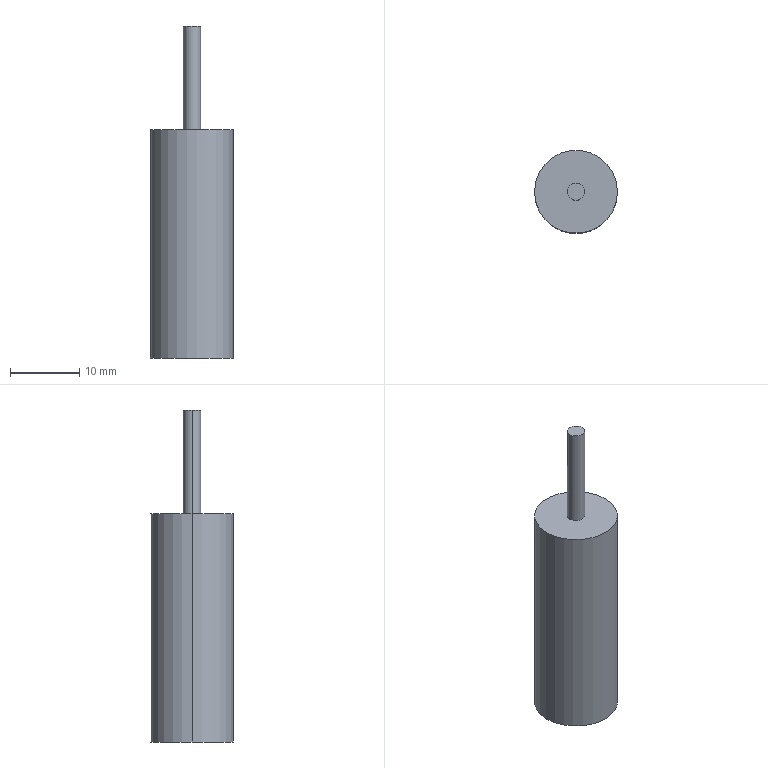Part | SolidWorks | features ICE 2 | 1 solid | 7 faces | box 12 x 12 x 48 mm | volume 3806 mm3 | cylinder 4 | plane 3 | commonest cylinder face diameters 2.5 x2 12 x2
STEP:
#1=CARTESIAN_POINT('',(1.25,0.,48.));
#2=VERTEX_POINT('',#1);
#3=CARTESIAN_POINT('',(-1.25,0.,48.));
#4=VERTEX_POINT('',#3);
#5=CARTESIAN_POINT('',(0.,0.,48.));
#6=DIRECTION('',(0.,0.,1.));
#7=DIRECTION('',(1.,0.,0.));
#8=AXIS2_PLACEMENT_3D('',#5,#6,#7);
#9=CIRCLE('',#8,1.25);
#10=EDGE_CURVE('',#2,#4,#9,.T.);
#11=ORIENTED_EDGE('',*,*,#10,.F.);
#12=CARTESIAN_POINT('',(1.25,0.,33.));
#13=VERTEX_POINT('',#12);
#14=CARTESIAN_POINT('',(1.25,0.,48.));
#15=DIRECTION('',(0.,0.,-1.));
#16=VECTOR('',#15,1000.);
#17=LINE('',#14,#16);
#18=EDGE_CURVE('',#2,#13,#17,.T.);
#19=ORIENTED_EDGE('',*,*,#18,.T.);
#20=CARTESIAN_POINT('',(-1.25,0.,33.));
#21=VERTEX_POINT('',#20);
#22=CARTESIAN_POINT('',(0.,0.,33.));
#23=DIRECTION('',(0.,0.,1.));
#24=DIRECTION('',(1.,0.,0.));
#25=AXIS2_PLACEMENT_3D('',#22,#23,#24);
#26=CIRCLE('',#25,1.25);
#27=EDGE_CURVE('',#13,#21,#26,.T.);
#28=ORIENTED_EDGE('',*,*,#27,.T.);
#29=CARTESIAN_POINT('',(-1.25,0.,48.));
#30=DIRECTION('',(0.,0.,-1.));
#31=VECTOR('',#30,1000.);
#32=LINE('',#29,#31);
#33=EDGE_CURVE('',#4,#21,#32,.T.);
#34=ORIENTED_EDGE('',*,*,#33,.F.);
#35=EDGE_LOOP('',(#11,#19,#28,#34));
#36=FACE_OUTER_BOUND('',#35,.T.);
#37=CARTESIAN_POINT('',(0.,0.,48.));
#38=DIRECTION('',(0.,0.,-1.));
#39=DIRECTION('',(-1.,0.,0.));
#40=AXIS2_PLACEMENT_3D('',#37,#38,#39);
#41=CYLINDRICAL_SURFACE('',#40,1.25);
#42=ADVANCED_FACE('',(#36),#41,.T.);
#43=CARTESIAN_POINT('',(6.,0.,33.));
#44=VERTEX_POINT('',#43);
#45=CARTESIAN_POINT('',(-6.,0.,33.));
#46=VERTEX_POINT('',#45);
#47=CARTESIAN_POINT('',(0.,0.,33.));
#48=DIRECTION('',(0.,0.,1.));
#49=DIRECTION('',(1.,0.,0.));
#50=AXIS2_PLACEMENT_3D('',#47,#48,#49);
#51=CIRCLE('',#50,6.);
#52=EDGE_CURVE('',#44,#46,#51,.T.);
#53=ORIENTED_EDGE('',*,*,#52,.F.);
#54=CARTESIAN_POINT('',(6.,0.,0.));
#55=VERTEX_POINT('',#54);
#56=CARTESIAN_POINT('',(6.,0.,33.));
#57=DIRECTION('',(0.,0.,-1.));
#58=VECTOR('',#57,1000.);
#59=LINE('',#56,#58);
#60=EDGE_CURVE('',#44,#55,#59,.T.);
#61=ORIENTED_EDGE('',*,*,#60,.T.);
#62=CARTESIAN_POINT('',(-6.,0.,0.));
#63=VERTEX_POINT('',#62);
#64=CARTESIAN_POINT('',(0.,0.,0.));
#65=DIRECTION('',(0.,0.,1.));
#66=DIRECTION('',(1.,0.,0.));
#67=AXIS2_PLACEMENT_3D('',#64,#65,#66);
#68=CIRCLE('',#67,6.);
#69=EDGE_CURVE('',#55,#63,#68,.T.);
#70=ORIENTED_EDGE('',*,*,#69,.T.);
#71=CARTESIAN_POINT('',(-6.,0.,33.));
#72=DIRECTION('',(0.,0.,-1.));
#73=VECTOR('',#72,1000.);
#74=LINE('',#71,#73);
#75=EDGE_CURVE('',#46,#63,#74,.T.);
#76=ORIENTED_EDGE('',*,*,#75,.F.);
#77=EDGE_LOOP('',(#53,#61,#70,#76));
#78=FACE_OUTER_BOUND('',#77,.T.);
#79=CARTESIAN_POINT('',(0.,0.,33.));
#80=DIRECTION('',(0.,0.,-1.));
#81=DIRECTION('',(-1.,0.,0.));
#82=AXIS2_PLACEMENT_3D('',#79,#80,#81);
#83=CYLINDRICAL_SURFACE('',#82,6.);
#84=ADVANCED_FACE('',(#78),#83,.T.);
#85=CARTESIAN_POINT('',(0.,0.,33.));
#86=DIRECTION('',(0.,0.,1.));
#87=DIRECTION('',(1.,0.,0.));
#88=AXIS2_PLACEMENT_3D('',#85,#86,#87);
#89=CIRCLE('',#88,6.);
#90=EDGE_CURVE('',#46,#44,#89,.T.);
#91=ORIENTED_EDGE('',*,*,#90,.T.);
#92=ORIENTED_EDGE('',*,*,#52,.T.);
#93=EDGE_LOOP('',(#91,#92));
#94=FACE_OUTER_BOUND('',#93,.T.);
#95=CARTESIAN_POINT('',(0.,0.,33.));
#96=DIRECTION('',(0.,0.,1.));
#97=DIRECTION('',(1.,0.,0.));
#98=AXIS2_PLACEMENT_3D('',#95,#96,#97);
#99=CIRCLE('',#98,1.25);
#100=EDGE_CURVE('',#21,#13,#99,.T.);
#101=ORIENTED_EDGE('',*,*,#100,.F.);
#102=ORIENTED_EDGE('',*,*,#27,.F.);
#103=EDGE_LOOP('',(#101,#102));
#104=FACE_BOUND('',#103,.T.);
#105=CARTESIAN_POINT('',(0.,0.,33.));
#106=DIRECTION('',(0.,0.,1.));
#107=DIRECTION('',(1.,0.,0.));
#108=AXIS2_PLACEMENT_3D('',#105,#106,#107);
#109=PLANE('',#108);
#110=ADVANCED_FACE('',(#94,#104),#109,.T.);
#111=ORIENTED_EDGE('',*,*,#60,.F.);
#112=ORIENTED_EDGE('',*,*,#90,.F.);
#113=ORIENTED_EDGE('',*,*,#75,.T.);
#114=CARTESIAN_POINT('',(0.,0.,0.));
#115=DIRECTION('',(0.,0.,1.));
#116=DIRECTION('',(1.,0.,0.));
#117=AXIS2_PLACEMENT_3D('',#114,#115,#116);
#118=CIRCLE('',#117,6.);
#119=EDGE_CURVE('',#63,#55,#118,.T.);
#120=ORIENTED_EDGE('',*,*,#119,.T.);
#121=EDGE_LOOP('',(#111,#112,#113,#120));
#122=FACE_OUTER_BOUND('',#121,.T.);
#123=CARTESIAN_POINT('',(0.,0.,33.));
#124=DIRECTION('',(0.,0.,-1.));
#125=DIRECTION('',(-1.,0.,0.));
#126=AXIS2_PLACEMENT_3D('',#123,#124,#125);
#127=CYLINDRICAL_SURFACE('',#126,6.);
#128=ADVANCED_FACE('',(#122),#127,.T.);
#129=ORIENTED_EDGE('',*,*,#119,.F.);
#130=ORIENTED_EDGE('',*,*,#69,.F.);
#131=EDGE_LOOP('',(#129,#130));
#132=FACE_OUTER_BOUND('',#131,.T.);
#133=CARTESIAN_POINT('',(0.,0.,0.));
#134=DIRECTION('',(0.,0.,1.));
#135=DIRECTION('',(1.,0.,0.));
#136=AXIS2_PLACEMENT_3D('',#133,#134,#135);
#137=PLANE('',#136);
#138=ADVANCED_FACE('',(#132),#137,.F.);
#139=ORIENTED_EDGE('',*,*,#18,.F.);
#140=CARTESIAN_POINT('',(0.,0.,48.));
#141=DIRECTION('',(0.,0.,1.));
#142=DIRECTION('',(1.,0.,0.));
#143=AXIS2_PLACEMENT_3D('',#140,#141,#142);
#144=CIRCLE('',#143,1.25);
#145=EDGE_CURVE('',#4,#2,#144,.T.);
#146=ORIENTED_EDGE('',*,*,#145,.F.);
#147=ORIENTED_EDGE('',*,*,#33,.T.);
#148=ORIENTED_EDGE('',*,*,#100,.T.);
#149=EDGE_LOOP('',(#139,#146,#147,#148));
#150=FACE_OUTER_BOUND('',#149,.T.);
#151=CARTESIAN_POINT('',(0.,0.,48.));
#152=DIRECTION('',(0.,0.,-1.));
#153=DIRECTION('',(-1.,0.,0.));
#154=AXIS2_PLACEMENT_3D('',#151,#152,#153);
#155=CYLINDRICAL_SURFACE('',#154,1.25);
#156=ADVANCED_FACE('',(#150),#155,.T.);
#157=ORIENTED_EDGE('',*,*,#145,.T.);
#158=ORIENTED_EDGE('',*,*,#10,.T.);
#159=EDGE_LOOP('',(#157,#158));
#160=FACE_OUTER_BOUND('',#159,.T.);
#161=CARTESIAN_POINT('',(0.,0.,48.));
#162=DIRECTION('',(0.,0.,1.));
#163=DIRECTION('',(1.,0.,0.));
#164=AXIS2_PLACEMENT_3D('',#161,#162,#163);
#165=PLANE('',#164);
#166=ADVANCED_FACE('',(#160),#165,.T.);
#167=CLOSED_SHELL('',(#42,#84,#110,#128,#138,#156,#166));
#168=MANIFOLD_SOLID_BREP('',#167);
#169=CARTESIAN_POINT('',(0.,0.,0.));
#170=DIRECTION('',(0.,0.,1.));
#171=DIRECTION('',(1.,0.,0.));
#172=AXIS2_PLACEMENT_3D('',#169,#170,#171);
#173=(LENGTH_UNIT()NAMED_UNIT(*)SI_UNIT(.MILLI.,.METRE.));
#174=UNCERTAINTY_MEASURE_WITH_UNIT(LENGTH_MEASURE(0.00001),#173,'','');
#175=(NAMED_UNIT(*)PLANE_ANGLE_UNIT()SI_UNIT($,.RADIAN.));
#176=(NAMED_UNIT(*)SI_UNIT($,.STERADIAN.)SOLID_ANGLE_UNIT());
#177=(GEOMETRIC_REPRESENTATION_CONTEXT(3)GLOBAL_UNCERTAINTY_ASSIGNED_CONTEXT((#174))GLOBAL_UNIT_ASSIGNED_CONTEXT((#173,#175,#176))REPRESENTATION_CONTEXT('',''));
#178=ADVANCED_BREP_SHAPE_REPRESENTATION('',(#168,#172),#177);